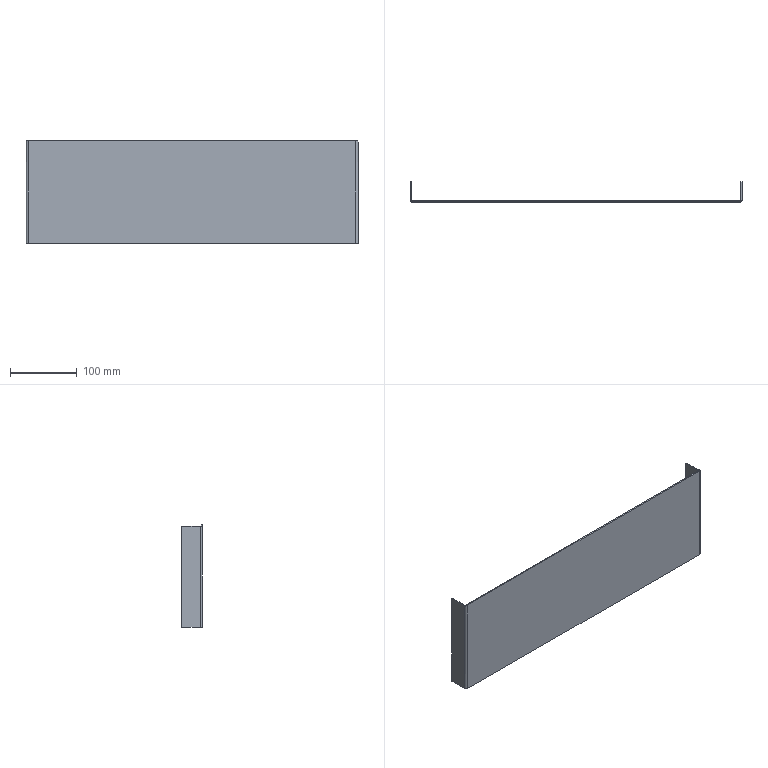Part | STEP file | 750038223 | 1 solid | 16 faces | box 496 x 30 x 153 mm | volume 126298 mm3 | plane 12 | cylinder 4 | commonest cylinder face diameters 3 x2 6 x2
STEP:
#1=CARTESIAN_POINT('',(-245.,1.5,-2.));
#2=VERTEX_POINT('',#1);
#3=CARTESIAN_POINT('',(-245.,1.5,-153.));
#4=VERTEX_POINT('',#3);
#5=CARTESIAN_POINT('',(-245.,1.5,0.));
#6=DIRECTION('',(0.,0.,-1.));
#7=VECTOR('',#6,1000.);
#8=LINE('',#5,#7);
#9=EDGE_CURVE('',#2,#4,#8,.T.);
#10=ORIENTED_EDGE('',*,*,#9,.F.);
#11=CARTESIAN_POINT('',(-247.598,1.5,-2.));
#12=VERTEX_POINT('',#11);
#13=CARTESIAN_POINT('',(248.,1.5,-2.));
#14=DIRECTION('',(1.,0.,0.));
#15=VECTOR('',#14,1000.);
#16=LINE('',#13,#15);
#17=EDGE_CURVE('',#12,#2,#16,.T.);
#18=ORIENTED_EDGE('',*,*,#17,.F.);
#19=CARTESIAN_POINT('',(-247.598,1.5,0.));
#20=VERTEX_POINT('',#19);
#21=CARTESIAN_POINT('',(-247.598,1.5,0.));
#22=DIRECTION('',(0.,0.,-1.));
#23=VECTOR('',#22,1000.);
#24=LINE('',#21,#23);
#25=EDGE_CURVE('',#20,#12,#24,.T.);
#26=ORIENTED_EDGE('',*,*,#25,.F.);
#27=CARTESIAN_POINT('',(247.598,1.5,0.));
#28=VERTEX_POINT('',#27);
#29=CARTESIAN_POINT('',(248.,1.5,0.));
#30=DIRECTION('',(-1.,0.,0.));
#31=VECTOR('',#30,1000.);
#32=LINE('',#29,#31);
#33=EDGE_CURVE('',#28,#20,#32,.T.);
#34=ORIENTED_EDGE('',*,*,#33,.F.);
#35=CARTESIAN_POINT('',(247.598,1.5,-2.));
#36=VERTEX_POINT('',#35);
#37=CARTESIAN_POINT('',(247.598,1.5,0.));
#38=DIRECTION('',(0.,0.,1.));
#39=VECTOR('',#38,1000.);
#40=LINE('',#37,#39);
#41=EDGE_CURVE('',#36,#28,#40,.T.);
#42=ORIENTED_EDGE('',*,*,#41,.F.);
#43=CARTESIAN_POINT('',(245.,1.5,-2.));
#44=VERTEX_POINT('',#43);
#45=CARTESIAN_POINT('',(248.,1.5,-2.));
#46=DIRECTION('',(1.,0.,0.));
#47=VECTOR('',#46,1000.);
#48=LINE('',#45,#47);
#49=EDGE_CURVE('',#44,#36,#48,.T.);
#50=ORIENTED_EDGE('',*,*,#49,.F.);
#51=CARTESIAN_POINT('',(245.,1.5,-153.));
#52=VERTEX_POINT('',#51);
#53=CARTESIAN_POINT('',(245.,1.5,0.));
#54=DIRECTION('',(0.,0.,1.));
#55=VECTOR('',#54,1000.);
#56=LINE('',#53,#55);
#57=EDGE_CURVE('',#52,#44,#56,.T.);
#58=ORIENTED_EDGE('',*,*,#57,.F.);
#59=CARTESIAN_POINT('',(248.,1.5,-153.));
#60=DIRECTION('',(1.,0.,0.));
#61=VECTOR('',#60,1000.);
#62=LINE('',#59,#61);
#63=EDGE_CURVE('',#4,#52,#62,.T.);
#64=ORIENTED_EDGE('',*,*,#63,.F.);
#65=EDGE_LOOP('',(#10,#18,#26,#34,#42,#50,#58,#64));
#66=FACE_OUTER_BOUND('',#65,.T.);
#67=CARTESIAN_POINT('',(248.,1.5,0.));
#68=DIRECTION('',(0.,-1.,0.));
#69=DIRECTION('',(0.,0.,-1.));
#70=AXIS2_PLACEMENT_3D('',#67,#68,#69);
#71=PLANE('',#70);
#72=ADVANCED_FACE('',(#66),#71,.F.);
#73=CARTESIAN_POINT('',(245.,0.,-153.));
#74=VERTEX_POINT('',#73);
#75=CARTESIAN_POINT('',(248.,3.,-153.));
#76=VERTEX_POINT('',#75);
#77=CARTESIAN_POINT('',(245.,3.,-153.));
#78=DIRECTION('',(0.,0.,1.));
#79=DIRECTION('',(-1.,0.,0.));
#80=AXIS2_PLACEMENT_3D('',#77,#78,#79);
#81=CIRCLE('',#80,3.);
#82=EDGE_CURVE('',#74,#76,#81,.T.);
#83=ORIENTED_EDGE('',*,*,#82,.F.);
#84=CARTESIAN_POINT('',(-245.,0.,-153.));
#85=VERTEX_POINT('',#84);
#86=CARTESIAN_POINT('',(248.,0.,-153.));
#87=DIRECTION('',(1.,0.,0.));
#88=VECTOR('',#87,1000.);
#89=LINE('',#86,#88);
#90=EDGE_CURVE('',#85,#74,#89,.T.);
#91=ORIENTED_EDGE('',*,*,#90,.F.);
#92=CARTESIAN_POINT('',(-248.,3.,-153.));
#93=VERTEX_POINT('',#92);
#94=CARTESIAN_POINT('',(-245.,3.,-153.));
#95=DIRECTION('',(0.,0.,1.));
#96=DIRECTION('',(-1.,0.,0.));
#97=AXIS2_PLACEMENT_3D('',#94,#95,#96);
#98=CIRCLE('',#97,3.);
#99=EDGE_CURVE('',#93,#85,#98,.T.);
#100=ORIENTED_EDGE('',*,*,#99,.F.);
#101=CARTESIAN_POINT('',(-248.,30.,-153.));
#102=VERTEX_POINT('',#101);
#103=CARTESIAN_POINT('',(-248.,30.,-153.));
#104=DIRECTION('',(0.,-1.,0.));
#105=VECTOR('',#104,1000.);
#106=LINE('',#103,#105);
#107=EDGE_CURVE('',#102,#93,#106,.T.);
#108=ORIENTED_EDGE('',*,*,#107,.F.);
#109=CARTESIAN_POINT('',(-246.5,30.,-153.));
#110=VERTEX_POINT('',#109);
#111=CARTESIAN_POINT('',(-248.,30.,-153.));
#112=DIRECTION('',(-1.,0.,0.));
#113=VECTOR('',#112,1000.);
#114=LINE('',#111,#113);
#115=EDGE_CURVE('',#110,#102,#114,.T.);
#116=ORIENTED_EDGE('',*,*,#115,.F.);
#117=CARTESIAN_POINT('',(-246.5,3.,-153.));
#118=VERTEX_POINT('',#117);
#119=CARTESIAN_POINT('',(-246.5,30.,-153.));
#120=DIRECTION('',(0.,1.,0.));
#121=VECTOR('',#120,1000.);
#122=LINE('',#119,#121);
#123=EDGE_CURVE('',#118,#110,#122,.T.);
#124=ORIENTED_EDGE('',*,*,#123,.F.);
#125=CARTESIAN_POINT('',(-245.,3.,-153.));
#126=DIRECTION('',(0.,0.,-1.));
#127=DIRECTION('',(-1.,0.,0.));
#128=AXIS2_PLACEMENT_3D('',#125,#126,#127);
#129=CIRCLE('',#128,1.5);
#130=EDGE_CURVE('',#4,#118,#129,.T.);
#131=ORIENTED_EDGE('',*,*,#130,.F.);
#132=ORIENTED_EDGE('',*,*,#63,.T.);
#133=CARTESIAN_POINT('',(246.5,3.,-153.));
#134=VERTEX_POINT('',#133);
#135=CARTESIAN_POINT('',(245.,3.,-153.));
#136=DIRECTION('',(0.,0.,-1.));
#137=DIRECTION('',(-1.,0.,0.));
#138=AXIS2_PLACEMENT_3D('',#135,#136,#137);
#139=CIRCLE('',#138,1.5);
#140=EDGE_CURVE('',#134,#52,#139,.T.);
#141=ORIENTED_EDGE('',*,*,#140,.F.);
#142=CARTESIAN_POINT('',(246.5,30.,-153.));
#143=VERTEX_POINT('',#142);
#144=CARTESIAN_POINT('',(246.5,30.,-153.));
#145=DIRECTION('',(0.,-1.,0.));
#146=VECTOR('',#145,1000.);
#147=LINE('',#144,#146);
#148=EDGE_CURVE('',#143,#134,#147,.T.);
#149=ORIENTED_EDGE('',*,*,#148,.F.);
#150=CARTESIAN_POINT('',(248.,30.,-153.));
#151=VERTEX_POINT('',#150);
#152=CARTESIAN_POINT('',(248.,30.,-153.));
#153=DIRECTION('',(1.,0.,0.));
#154=VECTOR('',#153,1000.);
#155=LINE('',#152,#154);
#156=EDGE_CURVE('',#143,#151,#155,.T.);
#157=ORIENTED_EDGE('',*,*,#156,.T.);
#158=CARTESIAN_POINT('',(248.,30.,-153.));
#159=DIRECTION('',(0.,1.,0.));
#160=VECTOR('',#159,1000.);
#161=LINE('',#158,#160);
#162=EDGE_CURVE('',#76,#151,#161,.T.);
#163=ORIENTED_EDGE('',*,*,#162,.F.);
#164=EDGE_LOOP('',(#83,#91,#100,#108,#116,#124,#131,#132,#141,#149,#157,#163));
#165=FACE_OUTER_BOUND('',#164,.T.);
#166=CARTESIAN_POINT('',(248.,30.,-153.));
#167=DIRECTION('',(0.,0.,1.));
#168=DIRECTION('',(1.,0.,0.));
#169=AXIS2_PLACEMENT_3D('',#166,#167,#168);
#170=PLANE('',#169);
#171=ADVANCED_FACE('',(#165),#170,.F.);
#172=ORIENTED_EDGE('',*,*,#9,.T.);
#173=ORIENTED_EDGE('',*,*,#130,.T.);
#174=CARTESIAN_POINT('',(-246.5,3.,-2.));
#175=VERTEX_POINT('',#174);
#176=CARTESIAN_POINT('',(-246.5,3.,0.));
#177=DIRECTION('',(0.,0.,-1.));
#178=VECTOR('',#177,1000.);
#179=LINE('',#176,#178);
#180=EDGE_CURVE('',#175,#118,#179,.T.);
#181=ORIENTED_EDGE('',*,*,#180,.F.);
#182=CARTESIAN_POINT('',(-245.,3.,-2.));
#183=DIRECTION('',(0.,0.,-1.));
#184=DIRECTION('',(-1.,0.,0.));
#185=AXIS2_PLACEMENT_3D('',#182,#183,#184);
#186=CIRCLE('',#185,1.5);
#187=EDGE_CURVE('',#2,#175,#186,.T.);
#188=ORIENTED_EDGE('',*,*,#187,.F.);
#189=EDGE_LOOP('',(#172,#173,#181,#188));
#190=FACE_OUTER_BOUND('',#189,.T.);
#191=CARTESIAN_POINT('',(-245.,3.,0.));
#192=DIRECTION('',(0.,0.,-1.));
#193=DIRECTION('',(-1.,0.,0.));
#194=AXIS2_PLACEMENT_3D('',#191,#192,#193);
#195=CYLINDRICAL_SURFACE('',#194,1.5);
#196=ADVANCED_FACE('',(#190),#195,.F.);
#197=CARTESIAN_POINT('',(-248.,30.,-2.));
#198=VERTEX_POINT('',#197);
#199=CARTESIAN_POINT('',(-248.,3.,-2.));
#200=VERTEX_POINT('',#199);
#201=CARTESIAN_POINT('',(-248.,0.,-2.));
#202=DIRECTION('',(0.,-1.,0.));
#203=VECTOR('',#202,1000.);
#204=LINE('',#201,#203);
#205=EDGE_CURVE('',#198,#200,#204,.T.);
#206=ORIENTED_EDGE('',*,*,#205,.T.);
#207=CARTESIAN_POINT('',(-245.,3.,-2.));
#208=DIRECTION('',(0.,0.,1.));
#209=DIRECTION('',(-1.,0.,0.));
#210=AXIS2_PLACEMENT_3D('',#207,#208,#209);
#211=CIRCLE('',#210,3.);
#212=EDGE_CURVE('',#200,#12,#211,.T.);
#213=ORIENTED_EDGE('',*,*,#212,.T.);
#214=ORIENTED_EDGE('',*,*,#17,.T.);
#215=ORIENTED_EDGE('',*,*,#187,.T.);
#216=CARTESIAN_POINT('',(-246.5,30.,-2.));
#217=VERTEX_POINT('',#216);
#218=CARTESIAN_POINT('',(-246.5,0.,-2.));
#219=DIRECTION('',(0.,1.,0.));
#220=VECTOR('',#219,1000.);
#221=LINE('',#218,#220);
#222=EDGE_CURVE('',#175,#217,#221,.T.);
#223=ORIENTED_EDGE('',*,*,#222,.T.);
#224=CARTESIAN_POINT('',(-248.,30.,-2.));
#225=DIRECTION('',(1.,0.,0.));
#226=VECTOR('',#225,1000.);
#227=LINE('',#224,#226);
#228=EDGE_CURVE('',#198,#217,#227,.T.);
#229=ORIENTED_EDGE('',*,*,#228,.F.);
#230=EDGE_LOOP('',(#206,#213,#214,#215,#223,#229));
#231=FACE_OUTER_BOUND('',#230,.T.);
#232=CARTESIAN_POINT('',(0.,0.,-2.));
#233=DIRECTION('',(0.,0.,1.));
#234=DIRECTION('',(1.,0.,0.));
#235=AXIS2_PLACEMENT_3D('',#232,#233,#234);
#236=PLANE('',#235);
#237=ADVANCED_FACE('',(#231),#236,.T.);
#238=CARTESIAN_POINT('',(-245.,0.,0.));
#239=VERTEX_POINT('',#238);
#240=CARTESIAN_POINT('',(-245.,0.,0.));
#241=DIRECTION('',(0.,0.,1.));
#242=VECTOR('',#241,1000.);
#243=LINE('',#240,#242);
#244=EDGE_CURVE('',#85,#239,#243,.T.);
#245=ORIENTED_EDGE('',*,*,#244,.T.);
#246=CARTESIAN_POINT('',(-245.,3.,0.));
#247=DIRECTION('',(0.,0.,-1.));
#248=DIRECTION('',(-1.,0.,0.));
#249=AXIS2_PLACEMENT_3D('',#246,#247,#248);
#250=CIRCLE('',#249,3.);
#251=EDGE_CURVE('',#239,#20,#250,.T.);
#252=ORIENTED_EDGE('',*,*,#251,.T.);
#253=ORIENTED_EDGE('',*,*,#25,.T.);
#254=ORIENTED_EDGE('',*,*,#212,.F.);
#255=CARTESIAN_POINT('',(-248.,3.,0.));
#256=DIRECTION('',(0.,0.,-1.));
#257=VECTOR('',#256,1000.);
#258=LINE('',#255,#257);
#259=EDGE_CURVE('',#200,#93,#258,.T.);
#260=ORIENTED_EDGE('',*,*,#259,.T.);
#261=ORIENTED_EDGE('',*,*,#99,.T.);
#262=EDGE_LOOP('',(#245,#252,#253,#254,#260,#261));
#263=FACE_OUTER_BOUND('',#262,.T.);
#264=CARTESIAN_POINT('',(-245.,3.,0.));
#265=DIRECTION('',(0.,0.,-1.));
#266=DIRECTION('',(-1.,0.,0.));
#267=AXIS2_PLACEMENT_3D('',#264,#265,#266);
#268=CYLINDRICAL_SURFACE('',#267,3.);
#269=ADVANCED_FACE('',(#263),#268,.T.);
#270=ORIENTED_EDGE('',*,*,#251,.F.);
#271=CARTESIAN_POINT('',(245.,0.,0.));
#272=VERTEX_POINT('',#271);
#273=CARTESIAN_POINT('',(-248.,0.,0.));
#274=DIRECTION('',(1.,0.,0.));
#275=VECTOR('',#274,1000.);
#276=LINE('',#273,#275);
#277=EDGE_CURVE('',#239,#272,#276,.T.);
#278=ORIENTED_EDGE('',*,*,#277,.T.);
#279=CARTESIAN_POINT('',(245.,3.,0.));
#280=DIRECTION('',(0.,0.,1.));
#281=DIRECTION('',(-1.,0.,0.));
#282=AXIS2_PLACEMENT_3D('',#279,#280,#281);
#283=CIRCLE('',#282,3.);
#284=EDGE_CURVE('',#272,#28,#283,.T.);
#285=ORIENTED_EDGE('',*,*,#284,.T.);
#286=ORIENTED_EDGE('',*,*,#33,.T.);
#287=EDGE_LOOP('',(#270,#278,#285,#286));
#288=FACE_OUTER_BOUND('',#287,.T.);
#289=CARTESIAN_POINT('',(-248.,0.,0.));
#290=DIRECTION('',(0.,0.,1.));
#291=DIRECTION('',(1.,0.,0.));
#292=AXIS2_PLACEMENT_3D('',#289,#290,#291);
#293=PLANE('',#292);
#294=ADVANCED_FACE('',(#288),#293,.T.);
#295=CARTESIAN_POINT('',(248.,3.,-2.));
#296=VERTEX_POINT('',#295);
#297=CARTESIAN_POINT('',(248.,3.,0.));
#298=DIRECTION('',(0.,0.,1.));
#299=VECTOR('',#298,1000.);
#300=LINE('',#297,#299);
#301=EDGE_CURVE('',#76,#296,#300,.T.);
#302=ORIENTED_EDGE('',*,*,#301,.T.);
#303=CARTESIAN_POINT('',(245.,3.,-2.));
#304=DIRECTION('',(0.,0.,-1.));
#305=DIRECTION('',(-1.,0.,0.));
#306=AXIS2_PLACEMENT_3D('',#303,#304,#305);
#307=CIRCLE('',#306,3.);
#308=EDGE_CURVE('',#296,#36,#307,.T.);
#309=ORIENTED_EDGE('',*,*,#308,.T.);
#310=ORIENTED_EDGE('',*,*,#41,.T.);
#311=ORIENTED_EDGE('',*,*,#284,.F.);
#312=CARTESIAN_POINT('',(245.,0.,0.));
#313=DIRECTION('',(0.,0.,-1.));
#314=VECTOR('',#313,1000.);
#315=LINE('',#312,#314);
#316=EDGE_CURVE('',#272,#74,#315,.T.);
#317=ORIENTED_EDGE('',*,*,#316,.T.);
#318=ORIENTED_EDGE('',*,*,#82,.T.);
#319=EDGE_LOOP('',(#302,#309,#310,#311,#317,#318));
#320=FACE_OUTER_BOUND('',#319,.T.);
#321=CARTESIAN_POINT('',(245.,3.,0.));
#322=DIRECTION('',(0.,0.,-1.));
#323=DIRECTION('',(-1.,0.,0.));
#324=AXIS2_PLACEMENT_3D('',#321,#322,#323);
#325=CYLINDRICAL_SURFACE('',#324,3.);
#326=ADVANCED_FACE('',(#320),#325,.T.);
#327=ORIENTED_EDGE('',*,*,#49,.T.);
#328=ORIENTED_EDGE('',*,*,#308,.F.);
#329=CARTESIAN_POINT('',(248.,30.,-2.));
#330=VERTEX_POINT('',#329);
#331=CARTESIAN_POINT('',(248.,0.,-2.));
#332=DIRECTION('',(0.,1.,0.));
#333=VECTOR('',#332,1000.);
#334=LINE('',#331,#333);
#335=EDGE_CURVE('',#296,#330,#334,.T.);
#336=ORIENTED_EDGE('',*,*,#335,.T.);
#337=CARTESIAN_POINT('',(246.5,30.,-2.));
#338=VERTEX_POINT('',#337);
#339=CARTESIAN_POINT('',(248.,30.,-2.));
#340=DIRECTION('',(-1.,0.,0.));
#341=VECTOR('',#340,1000.);
#342=LINE('',#339,#341);
#343=EDGE_CURVE('',#330,#338,#342,.T.);
#344=ORIENTED_EDGE('',*,*,#343,.T.);
#345=CARTESIAN_POINT('',(246.5,3.,-2.));
#346=VERTEX_POINT('',#345);
#347=CARTESIAN_POINT('',(246.5,0.,-2.));
#348=DIRECTION('',(0.,-1.,0.));
#349=VECTOR('',#348,1000.);
#350=LINE('',#347,#349);
#351=EDGE_CURVE('',#338,#346,#350,.T.);
#352=ORIENTED_EDGE('',*,*,#351,.T.);
#353=CARTESIAN_POINT('',(245.,3.,-2.));
#354=DIRECTION('',(0.,0.,-1.));
#355=DIRECTION('',(-1.,0.,0.));
#356=AXIS2_PLACEMENT_3D('',#353,#354,#355);
#357=CIRCLE('',#356,1.5);
#358=EDGE_CURVE('',#346,#44,#357,.T.);
#359=ORIENTED_EDGE('',*,*,#358,.T.);
#360=EDGE_LOOP('',(#327,#328,#336,#344,#352,#359));
#361=FACE_OUTER_BOUND('',#360,.T.);
#362=CARTESIAN_POINT('',(0.,0.,-2.));
#363=DIRECTION('',(0.,0.,1.));
#364=DIRECTION('',(1.,0.,0.));
#365=AXIS2_PLACEMENT_3D('',#362,#363,#364);
#366=PLANE('',#365);
#367=ADVANCED_FACE('',(#361),#366,.T.);
#368=CARTESIAN_POINT('',(246.5,3.,0.));
#369=DIRECTION('',(0.,0.,1.));
#370=VECTOR('',#369,1000.);
#371=LINE('',#368,#370);
#372=EDGE_CURVE('',#134,#346,#371,.T.);
#373=ORIENTED_EDGE('',*,*,#372,.F.);
#374=ORIENTED_EDGE('',*,*,#140,.T.);
#375=ORIENTED_EDGE('',*,*,#57,.T.);
#376=ORIENTED_EDGE('',*,*,#358,.F.);
#377=EDGE_LOOP('',(#373,#374,#375,#376));
#378=FACE_OUTER_BOUND('',#377,.T.);
#379=CARTESIAN_POINT('',(245.,3.,0.));
#380=DIRECTION('',(0.,0.,-1.));
#381=DIRECTION('',(-1.,0.,0.));
#382=AXIS2_PLACEMENT_3D('',#379,#380,#381);
#383=CYLINDRICAL_SURFACE('',#382,1.5);
#384=ADVANCED_FACE('',(#378),#383,.F.);
#385=ORIENTED_EDGE('',*,*,#162,.T.);
#386=CARTESIAN_POINT('',(248.,30.,0.));
#387=DIRECTION('',(0.,0.,1.));
#388=VECTOR('',#387,1000.);
#389=LINE('',#386,#388);
#390=EDGE_CURVE('',#151,#330,#389,.T.);
#391=ORIENTED_EDGE('',*,*,#390,.T.);
#392=ORIENTED_EDGE('',*,*,#335,.F.);
#393=ORIENTED_EDGE('',*,*,#301,.F.);
#394=EDGE_LOOP('',(#385,#391,#392,#393));
#395=FACE_OUTER_BOUND('',#394,.T.);
#396=CARTESIAN_POINT('',(248.,30.,0.));
#397=DIRECTION('',(1.,0.,0.));
#398=DIRECTION('',(0.,0.,-1.));
#399=AXIS2_PLACEMENT_3D('',#396,#397,#398);
#400=PLANE('',#399);
#401=ADVANCED_FACE('',(#395),#400,.T.);
#402=ORIENTED_EDGE('',*,*,#277,.F.);
#403=ORIENTED_EDGE('',*,*,#244,.F.);
#404=ORIENTED_EDGE('',*,*,#90,.T.);
#405=ORIENTED_EDGE('',*,*,#316,.F.);
#406=EDGE_LOOP('',(#402,#403,#404,#405));
#407=FACE_OUTER_BOUND('',#406,.T.);
#408=CARTESIAN_POINT('',(248.,0.,0.));
#409=DIRECTION('',(0.,-1.,0.));
#410=DIRECTION('',(0.,0.,-1.));
#411=AXIS2_PLACEMENT_3D('',#408,#409,#410);
#412=PLANE('',#411);
#413=ADVANCED_FACE('',(#407),#412,.T.);
#414=ORIENTED_EDGE('',*,*,#107,.T.);
#415=ORIENTED_EDGE('',*,*,#259,.F.);
#416=ORIENTED_EDGE('',*,*,#205,.F.);
#417=CARTESIAN_POINT('',(-248.,30.,0.));
#418=DIRECTION('',(0.,0.,-1.));
#419=VECTOR('',#418,1000.);
#420=LINE('',#417,#419);
#421=EDGE_CURVE('',#198,#102,#420,.T.);
#422=ORIENTED_EDGE('',*,*,#421,.T.);
#423=EDGE_LOOP('',(#414,#415,#416,#422));
#424=FACE_OUTER_BOUND('',#423,.T.);
#425=CARTESIAN_POINT('',(-248.,0.,0.));
#426=DIRECTION('',(-1.,0.,0.));
#427=DIRECTION('',(0.,0.,1.));
#428=AXIS2_PLACEMENT_3D('',#425,#426,#427);
#429=PLANE('',#428);
#430=ADVANCED_FACE('',(#424),#429,.T.);
#431=ORIENTED_EDGE('',*,*,#180,.T.);
#432=ORIENTED_EDGE('',*,*,#123,.T.);
#433=CARTESIAN_POINT('',(-246.5,30.,0.));
#434=DIRECTION('',(0.,0.,-1.));
#435=VECTOR('',#434,1000.);
#436=LINE('',#433,#435);
#437=EDGE_CURVE('',#217,#110,#436,.T.);
#438=ORIENTED_EDGE('',*,*,#437,.F.);
#439=ORIENTED_EDGE('',*,*,#222,.F.);
#440=EDGE_LOOP('',(#431,#432,#438,#439));
#441=FACE_OUTER_BOUND('',#440,.T.);
#442=CARTESIAN_POINT('',(-246.5,0.,0.));
#443=DIRECTION('',(-1.,0.,0.));
#444=DIRECTION('',(0.,0.,1.));
#445=AXIS2_PLACEMENT_3D('',#442,#443,#444);
#446=PLANE('',#445);
#447=ADVANCED_FACE('',(#441),#446,.F.);
#448=CARTESIAN_POINT('',(246.5,30.,0.));
#449=DIRECTION('',(0.,0.,1.));
#450=VECTOR('',#449,1000.);
#451=LINE('',#448,#450);
#452=EDGE_CURVE('',#143,#338,#451,.T.);
#453=ORIENTED_EDGE('',*,*,#452,.F.);
#454=ORIENTED_EDGE('',*,*,#148,.T.);
#455=ORIENTED_EDGE('',*,*,#372,.T.);
#456=ORIENTED_EDGE('',*,*,#351,.F.);
#457=EDGE_LOOP('',(#453,#454,#455,#456));
#458=FACE_OUTER_BOUND('',#457,.T.);
#459=CARTESIAN_POINT('',(246.5,30.,0.));
#460=DIRECTION('',(1.,0.,0.));
#461=DIRECTION('',(0.,0.,-1.));
#462=AXIS2_PLACEMENT_3D('',#459,#460,#461);
#463=PLANE('',#462);
#464=ADVANCED_FACE('',(#458),#463,.F.);
#465=ORIENTED_EDGE('',*,*,#390,.F.);
#466=ORIENTED_EDGE('',*,*,#156,.F.);
#467=ORIENTED_EDGE('',*,*,#452,.T.);
#468=ORIENTED_EDGE('',*,*,#343,.F.);
#469=EDGE_LOOP('',(#465,#466,#467,#468));
#470=FACE_OUTER_BOUND('',#469,.T.);
#471=CARTESIAN_POINT('',(248.,30.,0.));
#472=DIRECTION('',(0.,-1.,0.));
#473=DIRECTION('',(0.,0.,-1.));
#474=AXIS2_PLACEMENT_3D('',#471,#472,#473);
#475=PLANE('',#474);
#476=ADVANCED_FACE('',(#470),#475,.F.);
#477=ORIENTED_EDGE('',*,*,#115,.T.);
#478=ORIENTED_EDGE('',*,*,#421,.F.);
#479=ORIENTED_EDGE('',*,*,#228,.T.);
#480=ORIENTED_EDGE('',*,*,#437,.T.);
#481=EDGE_LOOP('',(#477,#478,#479,#480));
#482=FACE_OUTER_BOUND('',#481,.T.);
#483=CARTESIAN_POINT('',(-248.,30.,0.));
#484=DIRECTION('',(0.,1.,0.));
#485=DIRECTION('',(0.,0.,1.));
#486=AXIS2_PLACEMENT_3D('',#483,#484,#485);
#487=PLANE('',#486);
#488=ADVANCED_FACE('',(#482),#487,.T.);
#489=CLOSED_SHELL('',(#72,#171,#196,#237,#269,#294,#326,#367,#384,#401,#413,#430,#447,#464,#476,#488));
#490=MANIFOLD_SOLID_BREP('',#489);
#491=CARTESIAN_POINT('',(0.,0.,0.));
#492=DIRECTION('',(0.,0.,1.));
#493=DIRECTION('',(1.,0.,0.));
#494=AXIS2_PLACEMENT_3D('',#491,#492,#493);
#495=(LENGTH_UNIT()NAMED_UNIT(*)SI_UNIT(.MILLI.,.METRE.));
#496=UNCERTAINTY_MEASURE_WITH_UNIT(LENGTH_MEASURE(0.00001),#495,'','');
#497=(NAMED_UNIT(*)PLANE_ANGLE_UNIT()SI_UNIT($,.RADIAN.));
#498=(NAMED_UNIT(*)SI_UNIT($,.STERADIAN.)SOLID_ANGLE_UNIT());
#499=(GEOMETRIC_REPRESENTATION_CONTEXT(3)GLOBAL_UNCERTAINTY_ASSIGNED_CONTEXT((#496))GLOBAL_UNIT_ASSIGNED_CONTEXT((#495,#497,#498))REPRESENTATION_CONTEXT('',''));
#500=ADVANCED_BREP_SHAPE_REPRESENTATION('',(#490,#494),#499);